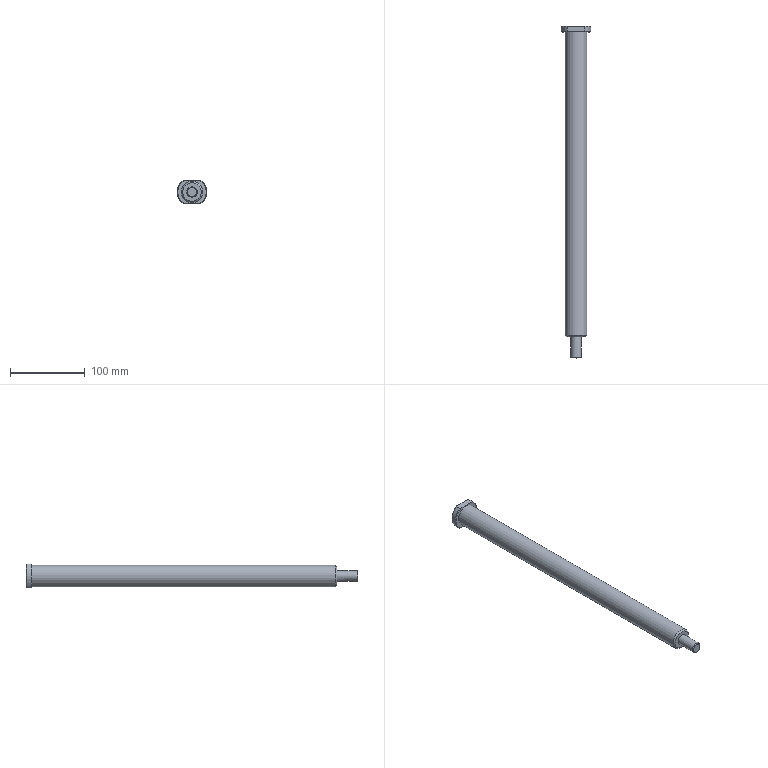Part | STEP file | HL4GZ-1.862.562 (swing arm long shaft) | 1 solid | 16 faces | box 40 x 444.5 x 32 mm | volume 282616 mm3 | plane 6 | cone 6 | cylinder 4 | commonest cylinder face diameters 40 x2 14 x1 29 x1
STEP:
#1=CARTESIAN_POINT('',(0.,0.,0.));
#2=DIRECTION('',(0.,0.,1.));
#3=DIRECTION('',(1.,0.,0.));
#4=AXIS2_PLACEMENT_3D('',#1,#2,#3);
#5=CARTESIAN_POINT('',(1836.876,25.5,-222.582));
#6=VERTEX_POINT('',#5);
#7=CARTESIAN_POINT('',(1838.63,26.5,-222.582));
#8=VERTEX_POINT('',#7);
#9=CARTESIAN_POINT('',(1836.876,25.5,-222.582));
#10=CARTESIAN_POINT('',(1837.451,25.81,-222.582));
#11=CARTESIAN_POINT('',(1838.035,26.143,-222.582));
#12=CARTESIAN_POINT('',(1838.63,26.5,-222.582));
#13=B_SPLINE_CURVE_WITH_KNOTS('',3,(#9,#10,#11,#12),.UNSPECIFIED.,.F.,.F.,(4,4),(0.,1.),.PIECEWISE_BEZIER_KNOTS.);
#14=CARTESIAN_POINT('',(1839.13,36.5,-222.582));
#15=DIRECTION('',(0.,0.,-1.));
#16=DIRECTION('',(1.,0.,0.));
#17=AXIS2_PLACEMENT_3D('',#14,#15,#16);
#18=PLANE('',#17);
#19=CARTESIAN_POINT('',(-2.253,11.));
#20=CARTESIAN_POINT('',(-1.678,10.69));
#21=CARTESIAN_POINT('',(-1.095,10.357));
#22=CARTESIAN_POINT('',(-0.5,10.));
#23=B_SPLINE_CURVE_WITH_KNOTS('',3,(#19,#20,#21,#22),.UNSPECIFIED.,.F.,.F.,(4,4),(0.,1.),.PIECEWISE_BEZIER_KNOTS.);
#24=(GEOMETRIC_REPRESENTATION_CONTEXT(2)PARAMETRIC_REPRESENTATION_CONTEXT()REPRESENTATION_CONTEXT('',''));
#25=DEFINITIONAL_REPRESENTATION('',(#23),#24);
#26=PCURVE('',#18,#25);
#27=CARTESIAN_POINT('',(1826.63,26.,-206.582));
#28=DIRECTION('',(0.,1.,0.));
#29=DIRECTION('',(-0.4067,0.,-0.9135));
#30=AXIS2_PLACEMENT_3D('',#27,#28,#29);
#31=CONICAL_SURFACE('',#30,19.5,0.7854);
#32=CARTESIAN_POINT('',(5.295,-0.5));
#33=CARTESIAN_POINT('',(5.294,-0.4859));
#34=CARTESIAN_POINT('',(5.291,-0.4576));
#35=CARTESIAN_POINT('',(5.288,-0.4149));
#36=CARTESIAN_POINT('',(5.284,-0.3719));
#37=CARTESIAN_POINT('',(5.281,-0.3287));
#38=CARTESIAN_POINT('',(5.277,-0.2851));
#39=CARTESIAN_POINT('',(5.274,-0.2412));
#40=CARTESIAN_POINT('',(5.271,-0.1971));
#41=CARTESIAN_POINT('',(5.267,-0.1526));
#42=CARTESIAN_POINT('',(5.264,-0.1079));
#43=CARTESIAN_POINT('',(5.26,-0.06289));
#44=CARTESIAN_POINT('',(5.257,-0.01758));
#45=CARTESIAN_POINT('',(5.254,0.02802));
#46=CARTESIAN_POINT('',(5.25,0.07391));
#47=CARTESIAN_POINT('',(5.247,0.1201));
#48=CARTESIAN_POINT('',(5.244,0.1666));
#49=CARTESIAN_POINT('',(5.24,0.2133));
#50=CARTESIAN_POINT('',(5.237,0.2604));
#51=CARTESIAN_POINT('',(5.234,0.3077));
#52=CARTESIAN_POINT('',(5.231,0.3553));
#53=CARTESIAN_POINT('',(5.227,0.4032));
#54=CARTESIAN_POINT('',(5.224,0.4515));
#55=CARTESIAN_POINT('',(5.222,0.4838));
#56=CARTESIAN_POINT('',(5.221,0.5));
#57=B_SPLINE_CURVE_WITH_KNOTS('',3,(#32,#33,#34,#35,#36,#37,#38,#39,#40,#41,#42,#43,#44,#45,#46,#47,#48,#49,#50,#51,#52,#53,#54,#55,#56),.UNSPECIFIED.,.F.,.F.,(4,1,1,1,1,1,1,1,1,1,1,1,1,1,1,1,1,1,1,1,1,1,4),(0.,0.04545,0.09091,0.1364,0.1818,0.2273,0.2727,0.3182,0.3636,0.4091,0.4545,0.5,0.5455,0.5909,0.6364,0.6818,0.7273,0.7727,0.8182,0.8636,0.9091,0.9545,1.),.QUASI_UNIFORM_KNOTS.);
#58=(GEOMETRIC_REPRESENTATION_CONTEXT(2)PARAMETRIC_REPRESENTATION_CONTEXT()REPRESENTATION_CONTEXT('',''));
#59=DEFINITIONAL_REPRESENTATION('',(#57),#58);
#60=PCURVE('',#31,#59);
#61=SURFACE_CURVE('',#13,(#26,#60),.PCURVE_S1.);
#62=EDGE_CURVE('',#6,#8,#61,.T.);
#63=ORIENTED_EDGE('',*,*,#62,.F.);
#64=CARTESIAN_POINT('',(1816.383,25.5,-222.582));
#65=VERTEX_POINT('',#64);
#66=CARTESIAN_POINT('',(1826.63,25.5,-222.582));
#67=DIRECTION('',(1.,0.,0.));
#68=VECTOR('',#67,1.);
#69=LINE('',#66,#68);
#70=CARTESIAN_POINT('',(-12.5,11.));
#71=DIRECTION('',(1.,0.));
#72=VECTOR('',#71,1.);
#73=LINE('',#70,#72);
#74=(GEOMETRIC_REPRESENTATION_CONTEXT(2)PARAMETRIC_REPRESENTATION_CONTEXT()REPRESENTATION_CONTEXT('',''));
#75=DEFINITIONAL_REPRESENTATION('',(#73),#74);
#76=PCURVE('',#18,#75);
#77=CARTESIAN_POINT('',(1826.63,25.5,-206.582));
#78=DIRECTION('',(0.,1.,0.));
#79=DIRECTION('',(0.4067,0.,0.9135));
#80=AXIS2_PLACEMENT_3D('',#77,#78,#79);
#81=PLANE('',#80);
#82=CARTESIAN_POINT('',(-14.617,6.508));
#83=DIRECTION('',(0.4067,0.9135));
#84=VECTOR('',#83,1.);
#85=LINE('',#82,#84);
#86=(GEOMETRIC_REPRESENTATION_CONTEXT(2)PARAMETRIC_REPRESENTATION_CONTEXT()REPRESENTATION_CONTEXT('',''));
#87=DEFINITIONAL_REPRESENTATION('',(#85),#86);
#88=PCURVE('',#81,#87);
#89=SURFACE_CURVE('',#69,(#76,#88),.PCURVE_S1.);
#90=EDGE_CURVE('',#65,#6,#89,.T.);
#91=ORIENTED_EDGE('',*,*,#90,.F.);
#92=CARTESIAN_POINT('',(1814.63,26.5,-222.582));
#93=VERTEX_POINT('',#92);
#94=CARTESIAN_POINT('',(1814.63,26.5,-222.582));
#95=CARTESIAN_POINT('',(1815.224,26.143,-222.582));
#96=CARTESIAN_POINT('',(1815.808,25.81,-222.582));
#97=CARTESIAN_POINT('',(1816.383,25.5,-222.582));
#98=B_SPLINE_CURVE_WITH_KNOTS('',3,(#94,#95,#96,#97),.UNSPECIFIED.,.F.,.F.,(4,4),(0.,1.),.PIECEWISE_BEZIER_KNOTS.);
#99=CARTESIAN_POINT('',(-24.5,10.));
#100=CARTESIAN_POINT('',(-23.905,10.357));
#101=CARTESIAN_POINT('',(-23.322,10.69));
#102=CARTESIAN_POINT('',(-22.747,11.));
#103=B_SPLINE_CURVE_WITH_KNOTS('',3,(#99,#100,#101,#102),.UNSPECIFIED.,.F.,.F.,(4,4),(0.,1.),.PIECEWISE_BEZIER_KNOTS.);
#104=(GEOMETRIC_REPRESENTATION_CONTEXT(2)PARAMETRIC_REPRESENTATION_CONTEXT()REPRESENTATION_CONTEXT('',''));
#105=DEFINITIONAL_REPRESENTATION('',(#103),#104);
#106=PCURVE('',#18,#105);
#107=CARTESIAN_POINT('',(1826.63,26.,-206.582));
#108=DIRECTION('',(0.,1.,0.));
#109=DIRECTION('',(-0.4067,0.,-0.9135));
#110=AXIS2_PLACEMENT_3D('',#107,#108,#109);
#111=CONICAL_SURFACE('',#110,19.5,0.7854);
#112=CARTESIAN_POINT('',(0.2246,0.5));
#113=CARTESIAN_POINT('',(0.2235,0.4838));
#114=CARTESIAN_POINT('',(0.2214,0.4515));
#115=CARTESIAN_POINT('',(0.2181,0.4032));
#116=CARTESIAN_POINT('',(0.2148,0.3553));
#117=CARTESIAN_POINT('',(0.2116,0.3077));
#118=CARTESIAN_POINT('',(0.2083,0.2604));
#119=CARTESIAN_POINT('',(0.205,0.2133));
#120=CARTESIAN_POINT('',(0.2017,0.1666));
#121=CARTESIAN_POINT('',(0.1983,0.1201));
#122=CARTESIAN_POINT('',(0.195,0.07391));
#123=CARTESIAN_POINT('',(0.1917,0.02802));
#124=CARTESIAN_POINT('',(0.1883,-0.01758));
#125=CARTESIAN_POINT('',(0.185,-0.06289));
#126=CARTESIAN_POINT('',(0.1816,-0.1079));
#127=CARTESIAN_POINT('',(0.1782,-0.1526));
#128=CARTESIAN_POINT('',(0.1748,-0.1971));
#129=CARTESIAN_POINT('',(0.1714,-0.2412));
#130=CARTESIAN_POINT('',(0.168,-0.2851));
#131=CARTESIAN_POINT('',(0.1646,-0.3287));
#132=CARTESIAN_POINT('',(0.1611,-0.3719));
#133=CARTESIAN_POINT('',(0.1577,-0.4149));
#134=CARTESIAN_POINT('',(0.1542,-0.4576));
#135=CARTESIAN_POINT('',(0.1519,-0.4859));
#136=CARTESIAN_POINT('',(0.1507,-0.5));
#137=B_SPLINE_CURVE_WITH_KNOTS('',3,(#112,#113,#114,#115,#116,#117,#118,#119,#120,#121,#122,#123,#124,#125,#126,#127,#128,#129,#130,#131,#132,#133,#134,#135,#136),.UNSPECIFIED.,.F.,.F.,(4,1,1,1,1,1,1,1,1,1,1,1,1,1,1,1,1,1,1,1,1,1,4),(0.,0.04545,0.09091,0.1364,0.1818,0.2273,0.2727,0.3182,0.3636,0.4091,0.4545,0.5,0.5455,0.5909,0.6364,0.6818,0.7273,0.7727,0.8182,0.8636,0.9091,0.9545,1.),.QUASI_UNIFORM_KNOTS.);
#138=(GEOMETRIC_REPRESENTATION_CONTEXT(2)PARAMETRIC_REPRESENTATION_CONTEXT()REPRESENTATION_CONTEXT('',''));
#139=DEFINITIONAL_REPRESENTATION('',(#137),#138);
#140=PCURVE('',#111,#139);
#141=SURFACE_CURVE('',#98,(#106,#140),.PCURVE_S1.);
#142=EDGE_CURVE('',#93,#65,#141,.T.);
#143=ORIENTED_EDGE('',*,*,#142,.F.);
#144=CARTESIAN_POINT('',(1814.63,32.5,-222.582));
#145=VERTEX_POINT('',#144);
#146=CARTESIAN_POINT('',(1814.63,25.5,-222.582));
#147=DIRECTION('',(0.,-1.,0.));
#148=VECTOR('',#147,1.);
#149=LINE('',#146,#148);
#150=CARTESIAN_POINT('',(-24.5,11.));
#151=DIRECTION('',(0.,1.));
#152=VECTOR('',#151,1.);
#153=LINE('',#150,#152);
#154=(GEOMETRIC_REPRESENTATION_CONTEXT(2)PARAMETRIC_REPRESENTATION_CONTEXT()REPRESENTATION_CONTEXT('',''));
#155=DEFINITIONAL_REPRESENTATION('',(#153),#154);
#156=PCURVE('',#18,#155);
#157=CARTESIAN_POINT('',(1826.63,25.5,-206.582));
#158=DIRECTION('',(0.,1.,0.));
#159=DIRECTION('',(-0.4067,0.,-0.9135));
#160=AXIS2_PLACEMENT_3D('',#157,#158,#159);
#161=CYLINDRICAL_SURFACE('',#160,20.);
#162=CARTESIAN_POINT('',(0.2246,0.));
#163=DIRECTION('',(0.,-1.));
#164=VECTOR('',#163,1.);
#165=LINE('',#162,#164);
#166=(GEOMETRIC_REPRESENTATION_CONTEXT(2)PARAMETRIC_REPRESENTATION_CONTEXT()REPRESENTATION_CONTEXT('',''));
#167=DEFINITIONAL_REPRESENTATION('',(#165),#166);
#168=PCURVE('',#161,#167);
#169=SURFACE_CURVE('',#149,(#156,#168),.PCURVE_S1.);
#170=EDGE_CURVE('',#145,#93,#169,.T.);
#171=ORIENTED_EDGE('',*,*,#170,.F.);
#172=CARTESIAN_POINT('',(1816.383,33.5,-222.582));
#173=VERTEX_POINT('',#172);
#174=CARTESIAN_POINT('',(1816.383,33.5,-222.582));
#175=CARTESIAN_POINT('',(1815.808,33.19,-222.582));
#176=CARTESIAN_POINT('',(1815.224,32.857,-222.582));
#177=CARTESIAN_POINT('',(1814.63,32.5,-222.582));
#178=B_SPLINE_CURVE_WITH_KNOTS('',3,(#174,#175,#176,#177),.UNSPECIFIED.,.F.,.F.,(4,4),(0.,1.),.PIECEWISE_BEZIER_KNOTS.);
#179=CARTESIAN_POINT('',(-22.747,3.));
#180=CARTESIAN_POINT('',(-23.322,3.31));
#181=CARTESIAN_POINT('',(-23.905,3.643));
#182=CARTESIAN_POINT('',(-24.5,4.));
#183=B_SPLINE_CURVE_WITH_KNOTS('',3,(#179,#180,#181,#182),.UNSPECIFIED.,.F.,.F.,(4,4),(0.,1.),.PIECEWISE_BEZIER_KNOTS.);
#184=(GEOMETRIC_REPRESENTATION_CONTEXT(2)PARAMETRIC_REPRESENTATION_CONTEXT()REPRESENTATION_CONTEXT('',''));
#185=DEFINITIONAL_REPRESENTATION('',(#183),#184);
#186=PCURVE('',#18,#185);
#187=CARTESIAN_POINT('',(1826.63,33.,-206.582));
#188=DIRECTION('',(0.,-1.,0.));
#189=DIRECTION('',(-0.4067,0.,-0.9135));
#190=AXIS2_PLACEMENT_3D('',#187,#188,#189);
#191=CONICAL_SURFACE('',#190,19.5,0.7854);
#192=CARTESIAN_POINT('',(6.132,-0.5));
#193=CARTESIAN_POINT('',(6.131,-0.4859));
#194=CARTESIAN_POINT('',(6.129,-0.4576));
#195=CARTESIAN_POINT('',(6.126,-0.4149));
#196=CARTESIAN_POINT('',(6.122,-0.3719));
#197=CARTESIAN_POINT('',(6.119,-0.3287));
#198=CARTESIAN_POINT('',(6.115,-0.2851));
#199=CARTESIAN_POINT('',(6.112,-0.2412));
#200=CARTESIAN_POINT('',(6.108,-0.1971));
#201=CARTESIAN_POINT('',(6.105,-0.1526));
#202=CARTESIAN_POINT('',(6.102,-0.1079));
#203=CARTESIAN_POINT('',(6.098,-0.06289));
#204=CARTESIAN_POINT('',(6.095,-0.01758));
#205=CARTESIAN_POINT('',(6.092,0.02802));
#206=CARTESIAN_POINT('',(6.088,0.07391));
#207=CARTESIAN_POINT('',(6.085,0.1201));
#208=CARTESIAN_POINT('',(6.082,0.1666));
#209=CARTESIAN_POINT('',(6.078,0.2133));
#210=CARTESIAN_POINT('',(6.075,0.2604));
#211=CARTESIAN_POINT('',(6.072,0.3077));
#212=CARTESIAN_POINT('',(6.068,0.3553));
#213=CARTESIAN_POINT('',(6.065,0.4032));
#214=CARTESIAN_POINT('',(6.062,0.4515));
#215=CARTESIAN_POINT('',(6.06,0.4838));
#216=CARTESIAN_POINT('',(6.059,0.5));
#217=B_SPLINE_CURVE_WITH_KNOTS('',3,(#192,#193,#194,#195,#196,#197,#198,#199,#200,#201,#202,#203,#204,#205,#206,#207,#208,#209,#210,#211,#212,#213,#214,#215,#216),.UNSPECIFIED.,.F.,.F.,(4,1,1,1,1,1,1,1,1,1,1,1,1,1,1,1,1,1,1,1,1,1,4),(0.,0.04545,0.09091,0.1364,0.1818,0.2273,0.2727,0.3182,0.3636,0.4091,0.4545,0.5,0.5455,0.5909,0.6364,0.6818,0.7273,0.7727,0.8182,0.8636,0.9091,0.9545,1.),.QUASI_UNIFORM_KNOTS.);
#218=(GEOMETRIC_REPRESENTATION_CONTEXT(2)PARAMETRIC_REPRESENTATION_CONTEXT()REPRESENTATION_CONTEXT('',''));
#219=DEFINITIONAL_REPRESENTATION('',(#217),#218);
#220=PCURVE('',#191,#219);
#221=SURFACE_CURVE('',#178,(#186,#220),.PCURVE_S1.);
#222=EDGE_CURVE('',#173,#145,#221,.T.);
#223=ORIENTED_EDGE('',*,*,#222,.F.);
#224=CARTESIAN_POINT('',(1836.876,33.5,-222.582));
#225=VERTEX_POINT('',#224);
#226=CARTESIAN_POINT('',(1826.63,33.5,-222.582));
#227=DIRECTION('',(1.,0.,0.));
#228=VECTOR('',#227,1.);
#229=LINE('',#226,#228);
#230=CARTESIAN_POINT('',(-12.5,3.));
#231=DIRECTION('',(1.,0.));
#232=VECTOR('',#231,1.);
#233=LINE('',#230,#232);
#234=(GEOMETRIC_REPRESENTATION_CONTEXT(2)PARAMETRIC_REPRESENTATION_CONTEXT()REPRESENTATION_CONTEXT('',''));
#235=DEFINITIONAL_REPRESENTATION('',(#233),#234);
#236=PCURVE('',#18,#235);
#237=CARTESIAN_POINT('',(1826.63,33.5,-206.582));
#238=DIRECTION('',(0.,1.,0.));
#239=DIRECTION('',(0.4067,0.,0.9135));
#240=AXIS2_PLACEMENT_3D('',#237,#238,#239);
#241=PLANE('',#240);
#242=CARTESIAN_POINT('',(-14.617,6.508));
#243=DIRECTION('',(0.4067,0.9135));
#244=VECTOR('',#243,1.);
#245=LINE('',#242,#244);
#246=(GEOMETRIC_REPRESENTATION_CONTEXT(2)PARAMETRIC_REPRESENTATION_CONTEXT()REPRESENTATION_CONTEXT('',''));
#247=DEFINITIONAL_REPRESENTATION('',(#245),#246);
#248=PCURVE('',#241,#247);
#249=SURFACE_CURVE('',#229,(#236,#248),.PCURVE_S1.);
#250=EDGE_CURVE('',#173,#225,#249,.T.);
#251=ORIENTED_EDGE('',*,*,#250,.T.);
#252=CARTESIAN_POINT('',(1838.63,32.5,-222.582));
#253=VERTEX_POINT('',#252);
#254=CARTESIAN_POINT('',(1838.63,32.5,-222.582));
#255=CARTESIAN_POINT('',(1838.035,32.857,-222.582));
#256=CARTESIAN_POINT('',(1837.451,33.19,-222.582));
#257=CARTESIAN_POINT('',(1836.876,33.5,-222.582));
#258=B_SPLINE_CURVE_WITH_KNOTS('',3,(#254,#255,#256,#257),.UNSPECIFIED.,.F.,.F.,(4,4),(0.,1.),.PIECEWISE_BEZIER_KNOTS.);
#259=CARTESIAN_POINT('',(-0.5,4.));
#260=CARTESIAN_POINT('',(-1.095,3.643));
#261=CARTESIAN_POINT('',(-1.678,3.31));
#262=CARTESIAN_POINT('',(-2.253,3.));
#263=B_SPLINE_CURVE_WITH_KNOTS('',3,(#259,#260,#261,#262),.UNSPECIFIED.,.F.,.F.,(4,4),(0.,1.),.PIECEWISE_BEZIER_KNOTS.);
#264=(GEOMETRIC_REPRESENTATION_CONTEXT(2)PARAMETRIC_REPRESENTATION_CONTEXT()REPRESENTATION_CONTEXT('',''));
#265=DEFINITIONAL_REPRESENTATION('',(#263),#264);
#266=PCURVE('',#18,#265);
#267=CARTESIAN_POINT('',(1826.63,33.,-206.582));
#268=DIRECTION('',(0.,-1.,0.));
#269=DIRECTION('',(-0.4067,0.,-0.9135));
#270=AXIS2_PLACEMENT_3D('',#267,#268,#269);
#271=CONICAL_SURFACE('',#270,19.5,0.7854);
#272=CARTESIAN_POINT('',(1.062,0.5));
#273=CARTESIAN_POINT('',(1.061,0.4838));
#274=CARTESIAN_POINT('',(1.059,0.4515));
#275=CARTESIAN_POINT('',(1.056,0.4032));
#276=CARTESIAN_POINT('',(1.053,0.3553));
#277=CARTESIAN_POINT('',(1.049,0.3077));
#278=CARTESIAN_POINT('',(1.046,0.2604));
#279=CARTESIAN_POINT('',(1.043,0.2133));
#280=CARTESIAN_POINT('',(1.039,0.1666));
#281=CARTESIAN_POINT('',(1.036,0.1201));
#282=CARTESIAN_POINT('',(1.033,0.07391));
#283=CARTESIAN_POINT('',(1.029,0.02802));
#284=CARTESIAN_POINT('',(1.026,-0.01758));
#285=CARTESIAN_POINT('',(1.023,-0.06289));
#286=CARTESIAN_POINT('',(1.019,-0.1079));
#287=CARTESIAN_POINT('',(1.016,-0.1526));
#288=CARTESIAN_POINT('',(1.013,-0.1971));
#289=CARTESIAN_POINT('',(1.009,-0.2412));
#290=CARTESIAN_POINT('',(1.006,-0.2851));
#291=CARTESIAN_POINT('',(1.002,-0.3287));
#292=CARTESIAN_POINT('',(0.9989,-0.3719));
#293=CARTESIAN_POINT('',(0.9954,-0.4149));
#294=CARTESIAN_POINT('',(0.992,-0.4576));
#295=CARTESIAN_POINT('',(0.9897,-0.4859));
#296=CARTESIAN_POINT('',(0.9885,-0.5));
#297=B_SPLINE_CURVE_WITH_KNOTS('',3,(#272,#273,#274,#275,#276,#277,#278,#279,#280,#281,#282,#283,#284,#285,#286,#287,#288,#289,#290,#291,#292,#293,#294,#295,#296),.UNSPECIFIED.,.F.,.F.,(4,1,1,1,1,1,1,1,1,1,1,1,1,1,1,1,1,1,1,1,1,1,4),(0.,0.04545,0.09091,0.1364,0.1818,0.2273,0.2727,0.3182,0.3636,0.4091,0.4545,0.5,0.5455,0.5909,0.6364,0.6818,0.7273,0.7727,0.8182,0.8636,0.9091,0.9545,1.),.QUASI_UNIFORM_KNOTS.);
#298=(GEOMETRIC_REPRESENTATION_CONTEXT(2)PARAMETRIC_REPRESENTATION_CONTEXT()REPRESENTATION_CONTEXT('',''));
#299=DEFINITIONAL_REPRESENTATION('',(#297),#298);
#300=PCURVE('',#271,#299);
#301=SURFACE_CURVE('',#258,(#266,#300),.PCURVE_S1.);
#302=EDGE_CURVE('',#253,#225,#301,.T.);
#303=ORIENTED_EDGE('',*,*,#302,.F.);
#304=CARTESIAN_POINT('',(1838.63,25.5,-222.582));
#305=DIRECTION('',(0.,1.,0.));
#306=VECTOR('',#305,1.);
#307=LINE('',#304,#306);
#308=CARTESIAN_POINT('',(-0.5,11.));
#309=DIRECTION('',(0.,-1.));
#310=VECTOR('',#309,1.);
#311=LINE('',#308,#310);
#312=(GEOMETRIC_REPRESENTATION_CONTEXT(2)PARAMETRIC_REPRESENTATION_CONTEXT()REPRESENTATION_CONTEXT('',''));
#313=DEFINITIONAL_REPRESENTATION('',(#311),#312);
#314=PCURVE('',#18,#313);
#315=CARTESIAN_POINT('',(1826.63,25.5,-206.582));
#316=DIRECTION('',(0.,1.,0.));
#317=DIRECTION('',(-0.4067,0.,-0.9135));
#318=AXIS2_PLACEMENT_3D('',#315,#316,#317);
#319=CYLINDRICAL_SURFACE('',#318,20.);
#320=CARTESIAN_POINT('',(5.221,0.));
#321=DIRECTION('',(0.,1.));
#322=VECTOR('',#321,1.);
#323=LINE('',#320,#322);
#324=(GEOMETRIC_REPRESENTATION_CONTEXT(2)PARAMETRIC_REPRESENTATION_CONTEXT()REPRESENTATION_CONTEXT('',''));
#325=DEFINITIONAL_REPRESENTATION('',(#323),#324);
#326=PCURVE('',#319,#325);
#327=SURFACE_CURVE('',#307,(#314,#326),.PCURVE_S1.);
#328=EDGE_CURVE('',#8,#253,#327,.T.);
#329=ORIENTED_EDGE('',*,*,#328,.F.);
#330=EDGE_LOOP('',(#63,#91,#143,#171,#223,#251,#303,#329));
#331=FACE_BOUND('',#330,.T.);
#332=ADVANCED_FACE('',(#331),#18,.T.);
#333=CARTESIAN_POINT('',(1838.63,26.5,-190.582));
#334=VERTEX_POINT('',#333);
#335=CARTESIAN_POINT('',(1836.876,25.5,-190.582));
#336=VERTEX_POINT('',#335);
#337=CARTESIAN_POINT('',(1838.63,26.5,-190.582));
#338=CARTESIAN_POINT('',(1838.035,26.143,-190.582));
#339=CARTESIAN_POINT('',(1837.451,25.81,-190.582));
#340=CARTESIAN_POINT('',(1836.876,25.5,-190.582));
#341=B_SPLINE_CURVE_WITH_KNOTS('',3,(#337,#338,#339,#340),.UNSPECIFIED.,.F.,.F.,(4,4),(0.,1.),.PIECEWISE_BEZIER_KNOTS.);
#342=CARTESIAN_POINT('',(1839.13,36.5,-190.582));
#343=DIRECTION('',(0.,0.,-1.));
#344=DIRECTION('',(1.,0.,0.));
#345=AXIS2_PLACEMENT_3D('',#342,#343,#344);
#346=PLANE('',#345);
#347=CARTESIAN_POINT('',(-0.5,10.));
#348=CARTESIAN_POINT('',(-1.095,10.357));
#349=CARTESIAN_POINT('',(-1.678,10.69));
#350=CARTESIAN_POINT('',(-2.253,11.));
#351=B_SPLINE_CURVE_WITH_KNOTS('',3,(#347,#348,#349,#350),.UNSPECIFIED.,.F.,.F.,(4,4),(0.,1.),.PIECEWISE_BEZIER_KNOTS.);
#352=(GEOMETRIC_REPRESENTATION_CONTEXT(2)PARAMETRIC_REPRESENTATION_CONTEXT()REPRESENTATION_CONTEXT('',''));
#353=DEFINITIONAL_REPRESENTATION('',(#351),#352);
#354=PCURVE('',#346,#353);
#355=CARTESIAN_POINT('',(3.366,0.5));
#356=CARTESIAN_POINT('',(3.365,0.4838));
#357=CARTESIAN_POINT('',(3.363,0.4515));
#358=CARTESIAN_POINT('',(3.36,0.4032));
#359=CARTESIAN_POINT('',(3.356,0.3553));
#360=CARTESIAN_POINT('',(3.353,0.3077));
#361=CARTESIAN_POINT('',(3.35,0.2604));
#362=CARTESIAN_POINT('',(3.347,0.2133));
#363=CARTESIAN_POINT('',(3.343,0.1666));
#364=CARTESIAN_POINT('',(3.34,0.1201));
#365=CARTESIAN_POINT('',(3.337,0.07391));
#366=CARTESIAN_POINT('',(3.333,0.02802));
#367=CARTESIAN_POINT('',(3.33,-0.01758));
#368=CARTESIAN_POINT('',(3.327,-0.06289));
#369=CARTESIAN_POINT('',(3.323,-0.1079));
#370=CARTESIAN_POINT('',(3.32,-0.1526));
#371=CARTESIAN_POINT('',(3.316,-0.1971));
#372=CARTESIAN_POINT('',(3.313,-0.2412));
#373=CARTESIAN_POINT('',(3.31,-0.2851));
#374=CARTESIAN_POINT('',(3.306,-0.3287));
#375=CARTESIAN_POINT('',(3.303,-0.3719));
#376=CARTESIAN_POINT('',(3.299,-0.4149));
#377=CARTESIAN_POINT('',(3.296,-0.4576));
#378=CARTESIAN_POINT('',(3.293,-0.4859));
#379=CARTESIAN_POINT('',(3.292,-0.5));
#380=B_SPLINE_CURVE_WITH_KNOTS('',3,(#355,#356,#357,#358,#359,#360,#361,#362,#363,#364,#365,#366,#367,#368,#369,#370,#371,#372,#373,#374,#375,#376,#377,#378,#379),.UNSPECIFIED.,.F.,.F.,(4,1,1,1,1,1,1,1,1,1,1,1,1,1,1,1,1,1,1,1,1,1,4),(0.,0.04545,0.09091,0.1364,0.1818,0.2273,0.2727,0.3182,0.3636,0.4091,0.4545,0.5,0.5455,0.5909,0.6364,0.6818,0.7273,0.7727,0.8182,0.8636,0.9091,0.9545,1.),.QUASI_UNIFORM_KNOTS.);
#381=(GEOMETRIC_REPRESENTATION_CONTEXT(2)PARAMETRIC_REPRESENTATION_CONTEXT()REPRESENTATION_CONTEXT('',''));
#382=DEFINITIONAL_REPRESENTATION('',(#380),#381);
#383=PCURVE('',#31,#382);
#384=SURFACE_CURVE('',#341,(#354,#383),.PCURVE_S1.);
#385=EDGE_CURVE('',#334,#336,#384,.T.);
#386=ORIENTED_EDGE('',*,*,#385,.F.);
#387=CARTESIAN_POINT('',(1838.63,32.5,-190.582));
#388=VERTEX_POINT('',#387);
#389=CARTESIAN_POINT('',(1838.63,25.5,-190.582));
#390=DIRECTION('',(0.,-1.,0.));
#391=VECTOR('',#390,1.);
#392=LINE('',#389,#391);
#393=CARTESIAN_POINT('',(-0.5,11.));
#394=DIRECTION('',(0.,1.));
#395=VECTOR('',#394,1.);
#396=LINE('',#393,#395);
#397=(GEOMETRIC_REPRESENTATION_CONTEXT(2)PARAMETRIC_REPRESENTATION_CONTEXT()REPRESENTATION_CONTEXT('',''));
#398=DEFINITIONAL_REPRESENTATION('',(#396),#397);
#399=PCURVE('',#346,#398);
#400=CARTESIAN_POINT('',(3.366,0.));
#401=DIRECTION('',(0.,-1.));
#402=VECTOR('',#401,1.);
#403=LINE('',#400,#402);
#404=(GEOMETRIC_REPRESENTATION_CONTEXT(2)PARAMETRIC_REPRESENTATION_CONTEXT()REPRESENTATION_CONTEXT('',''));
#405=DEFINITIONAL_REPRESENTATION('',(#403),#404);
#406=PCURVE('',#319,#405);
#407=SURFACE_CURVE('',#392,(#399,#406),.PCURVE_S1.);
#408=EDGE_CURVE('',#388,#334,#407,.T.);
#409=ORIENTED_EDGE('',*,*,#408,.F.);
#410=CARTESIAN_POINT('',(1836.876,33.5,-190.582));
#411=VERTEX_POINT('',#410);
#412=CARTESIAN_POINT('',(1836.876,33.5,-190.582));
#413=CARTESIAN_POINT('',(1837.451,33.19,-190.582));
#414=CARTESIAN_POINT('',(1838.035,32.857,-190.582));
#415=CARTESIAN_POINT('',(1838.63,32.5,-190.582));
#416=B_SPLINE_CURVE_WITH_KNOTS('',3,(#412,#413,#414,#415),.UNSPECIFIED.,.F.,.F.,(4,4),(0.,1.),.PIECEWISE_BEZIER_KNOTS.);
#417=CARTESIAN_POINT('',(-2.253,3.));
#418=CARTESIAN_POINT('',(-1.678,3.31));
#419=CARTESIAN_POINT('',(-1.095,3.643));
#420=CARTESIAN_POINT('',(-0.5,4.));
#421=B_SPLINE_CURVE_WITH_KNOTS('',3,(#417,#418,#419,#420),.UNSPECIFIED.,.F.,.F.,(4,4),(0.,1.),.PIECEWISE_BEZIER_KNOTS.);
#422=(GEOMETRIC_REPRESENTATION_CONTEXT(2)PARAMETRIC_REPRESENTATION_CONTEXT()REPRESENTATION_CONTEXT('',''));
#423=DEFINITIONAL_REPRESENTATION('',(#421),#422);
#424=PCURVE('',#346,#423);
#425=CARTESIAN_POINT('',(2.991,-0.5));
#426=CARTESIAN_POINT('',(2.99,-0.4859));
#427=CARTESIAN_POINT('',(2.987,-0.4576));
#428=CARTESIAN_POINT('',(2.984,-0.4149));
#429=CARTESIAN_POINT('',(2.98,-0.3719));
#430=CARTESIAN_POINT('',(2.977,-0.3287));
#431=CARTESIAN_POINT('',(2.974,-0.2851));
#432=CARTESIAN_POINT('',(2.97,-0.2412));
#433=CARTESIAN_POINT('',(2.967,-0.1971));
#434=CARTESIAN_POINT('',(2.963,-0.1526));
#435=CARTESIAN_POINT('',(2.96,-0.1079));
#436=CARTESIAN_POINT('',(2.957,-0.06289));
#437=CARTESIAN_POINT('',(2.953,-0.01758));
#438=CARTESIAN_POINT('',(2.95,0.02802));
#439=CARTESIAN_POINT('',(2.947,0.07391));
#440=CARTESIAN_POINT('',(2.943,0.1201));
#441=CARTESIAN_POINT('',(2.94,0.1666));
#442=CARTESIAN_POINT('',(2.937,0.2133));
#443=CARTESIAN_POINT('',(2.933,0.2604));
#444=CARTESIAN_POINT('',(2.93,0.3077));
#445=CARTESIAN_POINT('',(2.927,0.3553));
#446=CARTESIAN_POINT('',(2.923,0.4032));
#447=CARTESIAN_POINT('',(2.92,0.4515));
#448=CARTESIAN_POINT('',(2.918,0.4838));
#449=CARTESIAN_POINT('',(2.917,0.5));
#450=B_SPLINE_CURVE_WITH_KNOTS('',3,(#425,#426,#427,#428,#429,#430,#431,#432,#433,#434,#435,#436,#437,#438,#439,#440,#441,#442,#443,#444,#445,#446,#447,#448,#449),.UNSPECIFIED.,.F.,.F.,(4,1,1,1,1,1,1,1,1,1,1,1,1,1,1,1,1,1,1,1,1,1,4),(0.,0.04545,0.09091,0.1364,0.1818,0.2273,0.2727,0.3182,0.3636,0.4091,0.4545,0.5,0.5455,0.5909,0.6364,0.6818,0.7273,0.7727,0.8182,0.8636,0.9091,0.9545,1.),.QUASI_UNIFORM_KNOTS.);
#451=(GEOMETRIC_REPRESENTATION_CONTEXT(2)PARAMETRIC_REPRESENTATION_CONTEXT()REPRESENTATION_CONTEXT('',''));
#452=DEFINITIONAL_REPRESENTATION('',(#450),#451);
#453=PCURVE('',#271,#452);
#454=SURFACE_CURVE('',#416,(#424,#453),.PCURVE_S1.);
#455=EDGE_CURVE('',#411,#388,#454,.T.);
#456=ORIENTED_EDGE('',*,*,#455,.F.);
#457=CARTESIAN_POINT('',(1816.383,33.5,-190.582));
#458=VERTEX_POINT('',#457);
#459=CARTESIAN_POINT('',(1826.63,33.5,-190.582));
#460=DIRECTION('',(1.,0.,0.));
#461=VECTOR('',#460,1.);
#462=LINE('',#459,#461);
#463=CARTESIAN_POINT('',(-12.5,3.));
#464=DIRECTION('',(1.,0.));
#465=VECTOR('',#464,1.);
#466=LINE('',#463,#465);
#467=(GEOMETRIC_REPRESENTATION_CONTEXT(2)PARAMETRIC_REPRESENTATION_CONTEXT()REPRESENTATION_CONTEXT('',''));
#468=DEFINITIONAL_REPRESENTATION('',(#466),#467);
#469=PCURVE('',#346,#468);
#470=CARTESIAN_POINT('',(14.617,-6.508));
#471=DIRECTION('',(0.4067,0.9135));
#472=VECTOR('',#471,1.);
#473=LINE('',#470,#472);
#474=(GEOMETRIC_REPRESENTATION_CONTEXT(2)PARAMETRIC_REPRESENTATION_CONTEXT()REPRESENTATION_CONTEXT('',''));
#475=DEFINITIONAL_REPRESENTATION('',(#473),#474);
#476=PCURVE('',#241,#475);
#477=SURFACE_CURVE('',#462,(#469,#476),.PCURVE_S1.);
#478=EDGE_CURVE('',#458,#411,#477,.T.);
#479=ORIENTED_EDGE('',*,*,#478,.F.);
#480=CARTESIAN_POINT('',(1814.63,32.5,-190.582));
#481=VERTEX_POINT('',#480);
#482=CARTESIAN_POINT('',(1814.63,32.5,-190.582));
#483=CARTESIAN_POINT('',(1815.224,32.857,-190.582));
#484=CARTESIAN_POINT('',(1815.808,33.19,-190.582));
#485=CARTESIAN_POINT('',(1816.383,33.5,-190.582));
#486=B_SPLINE_CURVE_WITH_KNOTS('',3,(#482,#483,#484,#485),.UNSPECIFIED.,.F.,.F.,(4,4),(0.,1.),.PIECEWISE_BEZIER_KNOTS.);
#487=CARTESIAN_POINT('',(-24.5,4.));
#488=CARTESIAN_POINT('',(-23.905,3.643));
#489=CARTESIAN_POINT('',(-23.322,3.31));
#490=CARTESIAN_POINT('',(-22.747,3.));
#491=B_SPLINE_CURVE_WITH_KNOTS('',3,(#487,#488,#489,#490),.UNSPECIFIED.,.F.,.F.,(4,4),(0.,1.),.PIECEWISE_BEZIER_KNOTS.);
#492=(GEOMETRIC_REPRESENTATION_CONTEXT(2)PARAMETRIC_REPRESENTATION_CONTEXT()REPRESENTATION_CONTEXT('',''));
#493=DEFINITIONAL_REPRESENTATION('',(#491),#492);
#494=PCURVE('',#346,#493);
#495=CARTESIAN_POINT('',(4.204,0.5));
#496=CARTESIAN_POINT('',(4.203,0.4838));
#497=CARTESIAN_POINT('',(4.201,0.4515));
#498=CARTESIAN_POINT('',(4.197,0.4032));
#499=CARTESIAN_POINT('',(4.194,0.3553));
#500=CARTESIAN_POINT('',(4.191,0.3077));
#501=CARTESIAN_POINT('',(4.188,0.2604));
#502=CARTESIAN_POINT('',(4.184,0.2133));
#503=CARTESIAN_POINT('',(4.181,0.1666));
#504=CARTESIAN_POINT('',(4.178,0.1201));
#505=CARTESIAN_POINT('',(4.174,0.07391));
#506=CARTESIAN_POINT('',(4.171,0.02802));
#507=CARTESIAN_POINT('',(4.168,-0.01758));
#508=CARTESIAN_POINT('',(4.164,-0.06289));
#509=CARTESIAN_POINT('',(4.161,-0.1079));
#510=CARTESIAN_POINT('',(4.158,-0.1526));
#511=CARTESIAN_POINT('',(4.154,-0.1971));
#512=CARTESIAN_POINT('',(4.151,-0.2412));
#513=CARTESIAN_POINT('',(4.147,-0.2851));
#514=CARTESIAN_POINT('',(4.144,-0.3287));
#515=CARTESIAN_POINT('',(4.14,-0.3719));
#516=CARTESIAN_POINT('',(4.137,-0.4149));
#517=CARTESIAN_POINT('',(4.134,-0.4576));
#518=CARTESIAN_POINT('',(4.131,-0.4859));
#519=CARTESIAN_POINT('',(4.13,-0.5));
#520=B_SPLINE_CURVE_WITH_KNOTS('',3,(#495,#496,#497,#498,#499,#500,#501,#502,#503,#504,#505,#506,#507,#508,#509,#510,#511,#512,#513,#514,#515,#516,#517,#518,#519),.UNSPECIFIED.,.F.,.F.,(4,1,1,1,1,1,1,1,1,1,1,1,1,1,1,1,1,1,1,1,1,1,4),(0.,0.04545,0.09091,0.1364,0.1818,0.2273,0.2727,0.3182,0.3636,0.4091,0.4545,0.5,0.5455,0.5909,0.6364,0.6818,0.7273,0.7727,0.8182,0.8636,0.9091,0.9545,1.),.QUASI_UNIFORM_KNOTS.);
#521=(GEOMETRIC_REPRESENTATION_CONTEXT(2)PARAMETRIC_REPRESENTATION_CONTEXT()REPRESENTATION_CONTEXT('',''));
#522=DEFINITIONAL_REPRESENTATION('',(#520),#521);
#523=PCURVE('',#191,#522);
#524=SURFACE_CURVE('',#486,(#494,#523),.PCURVE_S1.);
#525=EDGE_CURVE('',#481,#458,#524,.T.);
#526=ORIENTED_EDGE('',*,*,#525,.F.);
#527=CARTESIAN_POINT('',(1814.63,26.5,-190.582));
#528=VERTEX_POINT('',#527);
#529=CARTESIAN_POINT('',(1814.63,25.5,-190.582));
#530=DIRECTION('',(0.,1.,0.));
#531=VECTOR('',#530,1.);
#532=LINE('',#529,#531);
#533=CARTESIAN_POINT('',(-24.5,11.));
#534=DIRECTION('',(0.,-1.));
#535=VECTOR('',#534,1.);
#536=LINE('',#533,#535);
#537=(GEOMETRIC_REPRESENTATION_CONTEXT(2)PARAMETRIC_REPRESENTATION_CONTEXT()REPRESENTATION_CONTEXT('',''));
#538=DEFINITIONAL_REPRESENTATION('',(#536),#537);
#539=PCURVE('',#346,#538);
#540=CARTESIAN_POINT('',(2.079,0.));
#541=DIRECTION('',(0.,1.));
#542=VECTOR('',#541,1.);
#543=LINE('',#540,#542);
#544=(GEOMETRIC_REPRESENTATION_CONTEXT(2)PARAMETRIC_REPRESENTATION_CONTEXT()REPRESENTATION_CONTEXT('',''));
#545=DEFINITIONAL_REPRESENTATION('',(#543),#544);
#546=PCURVE('',#161,#545);
#547=SURFACE_CURVE('',#532,(#539,#546),.PCURVE_S1.);
#548=EDGE_CURVE('',#528,#481,#547,.T.);
#549=ORIENTED_EDGE('',*,*,#548,.F.);
#550=CARTESIAN_POINT('',(1816.383,25.5,-190.582));
#551=VERTEX_POINT('',#550);
#552=CARTESIAN_POINT('',(1816.383,25.5,-190.582));
#553=CARTESIAN_POINT('',(1815.808,25.81,-190.582));
#554=CARTESIAN_POINT('',(1815.224,26.143,-190.582));
#555=CARTESIAN_POINT('',(1814.63,26.5,-190.582));
#556=B_SPLINE_CURVE_WITH_KNOTS('',3,(#552,#553,#554,#555),.UNSPECIFIED.,.F.,.F.,(4,4),(0.,1.),.PIECEWISE_BEZIER_KNOTS.);
#557=CARTESIAN_POINT('',(-22.747,11.));
#558=CARTESIAN_POINT('',(-23.322,10.69));
#559=CARTESIAN_POINT('',(-23.905,10.357));
#560=CARTESIAN_POINT('',(-24.5,10.));
#561=B_SPLINE_CURVE_WITH_KNOTS('',3,(#557,#558,#559,#560),.UNSPECIFIED.,.F.,.F.,(4,4),(0.,1.),.PIECEWISE_BEZIER_KNOTS.);
#562=(GEOMETRIC_REPRESENTATION_CONTEXT(2)PARAMETRIC_REPRESENTATION_CONTEXT()REPRESENTATION_CONTEXT('',''));
#563=DEFINITIONAL_REPRESENTATION('',(#561),#562);
#564=PCURVE('',#346,#563);
#565=CARTESIAN_POINT('',(2.153,-0.5));
#566=CARTESIAN_POINT('',(2.152,-0.4859));
#567=CARTESIAN_POINT('',(2.15,-0.4576));
#568=CARTESIAN_POINT('',(2.146,-0.4149));
#569=CARTESIAN_POINT('',(2.143,-0.3719));
#570=CARTESIAN_POINT('',(2.139,-0.3287));
#571=CARTESIAN_POINT('',(2.136,-0.2851));
#572=CARTESIAN_POINT('',(2.132,-0.2412));
#573=CARTESIAN_POINT('',(2.129,-0.1971));
#574=CARTESIAN_POINT('',(2.126,-0.1526));
#575=CARTESIAN_POINT('',(2.122,-0.1079));
#576=CARTESIAN_POINT('',(2.119,-0.06289));
#577=CARTESIAN_POINT('',(2.116,-0.01758));
#578=CARTESIAN_POINT('',(2.112,0.02802));
#579=CARTESIAN_POINT('',(2.109,0.07391));
#580=CARTESIAN_POINT('',(2.105,0.1201));
#581=CARTESIAN_POINT('',(2.102,0.1666));
#582=CARTESIAN_POINT('',(2.099,0.2133));
#583=CARTESIAN_POINT('',(2.096,0.2604));
#584=CARTESIAN_POINT('',(2.092,0.3077));
#585=CARTESIAN_POINT('',(2.089,0.3553));
#586=CARTESIAN_POINT('',(2.086,0.4032));
#587=CARTESIAN_POINT('',(2.082,0.4515));
#588=CARTESIAN_POINT('',(2.08,0.4838));
#589=CARTESIAN_POINT('',(2.079,0.5));
#590=B_SPLINE_CURVE_WITH_KNOTS('',3,(#565,#566,#567,#568,#569,#570,#571,#572,#573,#574,#575,#576,#577,#578,#579,#580,#581,#582,#583,#584,#585,#586,#587,#588,#589),.UNSPECIFIED.,.F.,.F.,(4,1,1,1,1,1,1,1,1,1,1,1,1,1,1,1,1,1,1,1,1,1,4),(0.,0.04545,0.09091,0.1364,0.1818,0.2273,0.2727,0.3182,0.3636,0.4091,0.4545,0.5,0.5455,0.5909,0.6364,0.6818,0.7273,0.7727,0.8182,0.8636,0.9091,0.9545,1.),.QUASI_UNIFORM_KNOTS.);
#591=(GEOMETRIC_REPRESENTATION_CONTEXT(2)PARAMETRIC_REPRESENTATION_CONTEXT()REPRESENTATION_CONTEXT('',''));
#592=DEFINITIONAL_REPRESENTATION('',(#590),#591);
#593=PCURVE('',#111,#592);
#594=SURFACE_CURVE('',#556,(#564,#593),.PCURVE_S1.);
#595=EDGE_CURVE('',#551,#528,#594,.T.);
#596=ORIENTED_EDGE('',*,*,#595,.F.);
#597=CARTESIAN_POINT('',(1826.63,25.5,-190.582));
#598=DIRECTION('',(-1.,0.,0.));
#599=VECTOR('',#598,1.);
#600=LINE('',#597,#599);
#601=CARTESIAN_POINT('',(-12.5,11.));
#602=DIRECTION('',(-1.,0.));
#603=VECTOR('',#602,1.);
#604=LINE('',#601,#603);
#605=(GEOMETRIC_REPRESENTATION_CONTEXT(2)PARAMETRIC_REPRESENTATION_CONTEXT()REPRESENTATION_CONTEXT('',''));
#606=DEFINITIONAL_REPRESENTATION('',(#604),#605);
#607=PCURVE('',#346,#606);
#608=CARTESIAN_POINT('',(14.617,-6.508));
#609=DIRECTION('',(-0.4067,-0.9135));
#610=VECTOR('',#609,1.);
#611=LINE('',#608,#610);
#612=(GEOMETRIC_REPRESENTATION_CONTEXT(2)PARAMETRIC_REPRESENTATION_CONTEXT()REPRESENTATION_CONTEXT('',''));
#613=DEFINITIONAL_REPRESENTATION('',(#611),#612);
#614=PCURVE('',#81,#613);
#615=SURFACE_CURVE('',#600,(#607,#614),.PCURVE_S1.);
#616=EDGE_CURVE('',#336,#551,#615,.T.);
#617=ORIENTED_EDGE('',*,*,#616,.F.);
#618=EDGE_LOOP('',(#386,#409,#456,#479,#526,#549,#596,#617));
#619=FACE_BOUND('',#618,.T.);
#620=ADVANCED_FACE('',(#619),#346,.F.);
#621=CARTESIAN_POINT('',(1832.527,25.5,-193.336));
#622=VERTEX_POINT('',#621);
#623=CARTESIAN_POINT('',(1826.63,25.5,-206.582));
#624=DIRECTION('',(0.,-1.,0.));
#625=DIRECTION('',(-0.4067,0.,-0.9135));
#626=AXIS2_PLACEMENT_3D('',#623,#624,#625);
#627=CIRCLE('',#626,14.5);
#628=CARTESIAN_POINT('',(1826.63,25.5,-206.582));
#629=DIRECTION('',(0.,-1.,0.));
#630=DIRECTION('',(-0.4067,0.,-0.9135));
#631=AXIS2_PLACEMENT_3D('',#628,#629,#630);
#632=CYLINDRICAL_SURFACE('',#631,14.5);
#633=CARTESIAN_POINT('',(0.,0.));
#634=DIRECTION('',(1.,0.));
#635=VECTOR('',#634,1.);
#636=LINE('',#633,#635);
#637=(GEOMETRIC_REPRESENTATION_CONTEXT(2)PARAMETRIC_REPRESENTATION_CONTEXT()REPRESENTATION_CONTEXT('',''));
#638=DEFINITIONAL_REPRESENTATION('',(#636),#637);
#639=PCURVE('',#632,#638);
#640=CARTESIAN_POINT('',(-14.5,0.));
#641=CARTESIAN_POINT('',(-14.5,25.115));
#642=CARTESIAN_POINT('',(7.25,12.557));
#643=CARTESIAN_POINT('',(29.,0.));
#644=CARTESIAN_POINT('',(7.25,-12.557));
#645=CARTESIAN_POINT('',(-14.5,-25.115));
#646=CARTESIAN_POINT('',(-14.5,0.));
#647=(BOUNDED_CURVE()B_SPLINE_CURVE(2,(#640,#641,#642,#643,#644,#645,#646),.UNSPECIFIED.,.T.,.F.)B_SPLINE_CURVE_WITH_KNOTS((1,2,2,2,2,1),(-2.094,0.,2.094,4.189,6.283,8.378),.UNSPECIFIED.)CURVE()GEOMETRIC_REPRESENTATION_ITEM()RATIONAL_B_SPLINE_CURVE((1.,0.5,1.,0.5,1.,0.5,1.))REPRESENTATION_ITEM(''));
#648=(GEOMETRIC_REPRESENTATION_CONTEXT(2)PARAMETRIC_REPRESENTATION_CONTEXT()REPRESENTATION_CONTEXT('',''));
#649=DEFINITIONAL_REPRESENTATION('',(#647),#648);
#650=PCURVE('',#81,#649);
#651=SURFACE_CURVE('',#627,(#639,#650),.PCURVE_S1.);
#652=EDGE_CURVE('',#622,#622,#651,.T.);
#653=ORIENTED_EDGE('',*,*,#652,.T.);
#654=CARTESIAN_POINT('',(1832.527,-380.5,-193.336));
#655=VERTEX_POINT('',#654);
#656=CARTESIAN_POINT('',(1832.527,25.5,-193.336));
#657=CARTESIAN_POINT('',(1832.527,-380.5,-193.336));
#658=B_SPLINE_CURVE_WITH_KNOTS('',1,(#656,#657),.UNSPECIFIED.,.F.,.F.,(2,2),(0.,406.),.PIECEWISE_BEZIER_KNOTS.);
#659=CARTESIAN_POINT('',(9.425,0.));
#660=DIRECTION('',(0.,1.));
#661=VECTOR('',#660,1.);
#662=LINE('',#659,#661);
#663=(GEOMETRIC_REPRESENTATION_CONTEXT(2)PARAMETRIC_REPRESENTATION_CONTEXT()REPRESENTATION_CONTEXT('',''));
#664=DEFINITIONAL_REPRESENTATION('',(#662),#663);
#665=PCURVE('',#632,#664);
#666=CARTESIAN_POINT('',(3.142,0.));
#667=DIRECTION('',(0.,1.));
#668=VECTOR('',#667,1.);
#669=LINE('',#666,#668);
#670=(GEOMETRIC_REPRESENTATION_CONTEXT(2)PARAMETRIC_REPRESENTATION_CONTEXT()REPRESENTATION_CONTEXT('',''));
#671=DEFINITIONAL_REPRESENTATION('',(#669),#670);
#672=PCURVE('',#632,#671);
#673=SEAM_CURVE('',#658,(#665,#672),.PCURVE_S1.);
#674=EDGE_CURVE('',#622,#655,#673,.T.);
#675=ORIENTED_EDGE('',*,*,#674,.T.);
#676=CARTESIAN_POINT('',(1826.63,-380.5,-206.582));
#677=DIRECTION('',(0.,-1.,0.));
#678=DIRECTION('',(-0.4067,0.,-0.9135));
#679=AXIS2_PLACEMENT_3D('',#676,#677,#678);
#680=CIRCLE('',#679,14.5);
#681=CARTESIAN_POINT('',(0.,406.));
#682=DIRECTION('',(1.,0.));
#683=VECTOR('',#682,1.);
#684=LINE('',#681,#683);
#685=(GEOMETRIC_REPRESENTATION_CONTEXT(2)PARAMETRIC_REPRESENTATION_CONTEXT()REPRESENTATION_CONTEXT('',''));
#686=DEFINITIONAL_REPRESENTATION('',(#684),#685);
#687=PCURVE('',#632,#686);
#688=CARTESIAN_POINT('',(1826.63,-381.5,-206.582));
#689=DIRECTION('',(0.,1.,0.));
#690=DIRECTION('',(-0.4067,0.,-0.9135));
#691=AXIS2_PLACEMENT_3D('',#688,#689,#690);
#692=CONICAL_SURFACE('',#691,13.5,0.7854);
#693=CARTESIAN_POINT('',(12.566,1.));
#694=DIRECTION('',(-1.,0.));
#695=VECTOR('',#694,1.);
#696=LINE('',#693,#695);
#697=(GEOMETRIC_REPRESENTATION_CONTEXT(2)PARAMETRIC_REPRESENTATION_CONTEXT()REPRESENTATION_CONTEXT('',''));
#698=DEFINITIONAL_REPRESENTATION('',(#696),#697);
#699=PCURVE('',#692,#698);
#700=SURFACE_CURVE('',#680,(#687,#699),.PCURVE_S1.);
#701=EDGE_CURVE('',#655,#655,#700,.T.);
#702=ORIENTED_EDGE('',*,*,#701,.F.);
#703=ORIENTED_EDGE('',*,*,#674,.F.);
#704=EDGE_LOOP('',(#653,#675,#702,#703));
#705=FACE_BOUND('',#704,.T.);
#706=ADVANCED_FACE('',(#705),#632,.T.);
#707=CARTESIAN_POINT('',(1824.189,-411.,-212.064));
#708=VERTEX_POINT('',#707);
#709=CARTESIAN_POINT('',(1826.63,-411.,-206.582));
#710=DIRECTION('',(0.,1.,0.));
#711=DIRECTION('',(0.4067,0.,0.9135));
#712=AXIS2_PLACEMENT_3D('',#709,#710,#711);
#713=CIRCLE('',#712,6.);
#714=CARTESIAN_POINT('',(1826.63,-411.,-206.582));
#715=DIRECTION('',(0.,1.,0.));
#716=DIRECTION('',(0.4067,0.,0.9135));
#717=AXIS2_PLACEMENT_3D('',#714,#715,#716);
#718=PLANE('',#717);
#719=CARTESIAN_POINT('',(0.,0.));
#720=DIRECTION('',(1.,0.));
#721=AXIS2_PLACEMENT_2D('',#719,#720);
#722=CIRCLE('',#721,6.);
#723=(GEOMETRIC_REPRESENTATION_CONTEXT(2)PARAMETRIC_REPRESENTATION_CONTEXT()REPRESENTATION_CONTEXT('',''));
#724=DEFINITIONAL_REPRESENTATION('',(#722),#723);
#725=PCURVE('',#718,#724);
#726=CARTESIAN_POINT('',(1826.63,-410.5,-206.582));
#727=DIRECTION('',(0.,1.,0.));
#728=DIRECTION('',(0.4067,0.,0.9135));
#729=AXIS2_PLACEMENT_3D('',#726,#727,#728);
#730=CONICAL_SURFACE('',#729,6.5,0.7854);
#731=CARTESIAN_POINT('',(0.,-0.5));
#732=DIRECTION('',(1.,0.));
#733=VECTOR('',#732,1.);
#734=LINE('',#731,#733);
#735=(GEOMETRIC_REPRESENTATION_CONTEXT(2)PARAMETRIC_REPRESENTATION_CONTEXT()REPRESENTATION_CONTEXT('',''));
#736=DEFINITIONAL_REPRESENTATION('',(#734),#735);
#737=PCURVE('',#730,#736);
#738=SURFACE_CURVE('',#713,(#725,#737),.PCURVE_S1.);
#739=EDGE_CURVE('',#708,#708,#738,.T.);
#740=ORIENTED_EDGE('',*,*,#739,.F.);
#741=EDGE_LOOP('',(#740));
#742=FACE_BOUND('',#741,.T.);
#743=ADVANCED_FACE('',(#742),#718,.F.);
#744=ORIENTED_EDGE('',*,*,#739,.T.);
#745=CARTESIAN_POINT('',(1823.782,-410.,-212.977));
#746=VERTEX_POINT('',#745);
#747=CARTESIAN_POINT('',(1824.189,-411.,-212.064));
#748=CARTESIAN_POINT('',(1823.782,-410.,-212.977));
#749=B_SPLINE_CURVE_WITH_KNOTS('',1,(#747,#748),.UNSPECIFIED.,.F.,.F.,(2,2),(-0.7071,0.7071),.PIECEWISE_BEZIER_KNOTS.);
#750=CARTESIAN_POINT('',(9.425,0.));
#751=DIRECTION('',(0.,1.));
#752=VECTOR('',#751,1.);
#753=LINE('',#750,#752);
#754=(GEOMETRIC_REPRESENTATION_CONTEXT(2)PARAMETRIC_REPRESENTATION_CONTEXT()REPRESENTATION_CONTEXT('',''));
#755=DEFINITIONAL_REPRESENTATION('',(#753),#754);
#756=PCURVE('',#730,#755);
#757=CARTESIAN_POINT('',(3.142,0.));
#758=DIRECTION('',(0.,1.));
#759=VECTOR('',#758,1.);
#760=LINE('',#757,#759);
#761=(GEOMETRIC_REPRESENTATION_CONTEXT(2)PARAMETRIC_REPRESENTATION_CONTEXT()REPRESENTATION_CONTEXT('',''));
#762=DEFINITIONAL_REPRESENTATION('',(#760),#761);
#763=PCURVE('',#730,#762);
#764=SEAM_CURVE('',#749,(#756,#763),.PCURVE_S1.);
#765=EDGE_CURVE('',#708,#746,#764,.T.);
#766=ORIENTED_EDGE('',*,*,#765,.T.);
#767=CARTESIAN_POINT('',(1819.782,-410.,-205.127));
#768=VERTEX_POINT('',#767);
#769=CARTESIAN_POINT('',(1826.63,-410.,-206.582));
#770=DIRECTION('',(0.,-1.,0.));
#771=DIRECTION('',(0.4067,0.,0.9135));
#772=AXIS2_PLACEMENT_3D('',#769,#770,#771);
#773=CIRCLE('',#772,7.);
#774=CARTESIAN_POINT('',(12.566,0.5));
#775=DIRECTION('',(-1.,0.));
#776=VECTOR('',#775,1.);
#777=LINE('',#774,#776);
#778=(GEOMETRIC_REPRESENTATION_CONTEXT(2)PARAMETRIC_REPRESENTATION_CONTEXT()REPRESENTATION_CONTEXT('',''));
#779=DEFINITIONAL_REPRESENTATION('',(#777),#778);
#780=PCURVE('',#730,#779);
#781=CARTESIAN_POINT('',(1826.63,-392.,-206.582));
#782=DIRECTION('',(0.,-1.,0.));
#783=DIRECTION('',(0.4067,0.,0.9135));
#784=AXIS2_PLACEMENT_3D('',#781,#782,#783);
#785=CYLINDRICAL_SURFACE('',#784,7.);
#786=CARTESIAN_POINT('',(0.,18.));
#787=DIRECTION('',(1.,0.));
#788=VECTOR('',#787,1.);
#789=LINE('',#786,#788);
#790=(GEOMETRIC_REPRESENTATION_CONTEXT(2)PARAMETRIC_REPRESENTATION_CONTEXT()REPRESENTATION_CONTEXT('',''));
#791=DEFINITIONAL_REPRESENTATION('',(#789),#790);
#792=PCURVE('',#785,#791);
#793=SURFACE_CURVE('',#773,(#780,#792),.PCURVE_S1.);
#794=EDGE_CURVE('',#746,#768,#793,.T.);
#795=ORIENTED_EDGE('',*,*,#794,.T.);
#796=CARTESIAN_POINT('',(1826.63,-410.,-206.582));
#797=DIRECTION('',(0.,-1.,0.));
#798=DIRECTION('',(0.4067,0.,0.9135));
#799=AXIS2_PLACEMENT_3D('',#796,#797,#798);
#800=CIRCLE('',#799,7.);
#801=CARTESIAN_POINT('',(6.283,0.5));
#802=DIRECTION('',(-1.,0.));
#803=VECTOR('',#802,1.);
#804=LINE('',#801,#803);
#805=(GEOMETRIC_REPRESENTATION_CONTEXT(2)PARAMETRIC_REPRESENTATION_CONTEXT()REPRESENTATION_CONTEXT('',''));
#806=DEFINITIONAL_REPRESENTATION('',(#804),#805);
#807=PCURVE('',#730,#806);
#808=CARTESIAN_POINT('',(0.,18.));
#809=DIRECTION('',(1.,0.));
#810=VECTOR('',#809,1.);
#811=LINE('',#808,#810);
#812=(GEOMETRIC_REPRESENTATION_CONTEXT(2)PARAMETRIC_REPRESENTATION_CONTEXT()REPRESENTATION_CONTEXT('',''));
#813=DEFINITIONAL_REPRESENTATION('',(#811),#812);
#814=PCURVE('',#785,#813);
#815=SURFACE_CURVE('',#800,(#807,#814),.PCURVE_S1.);
#816=EDGE_CURVE('',#768,#746,#815,.T.);
#817=ORIENTED_EDGE('',*,*,#816,.T.);
#818=ORIENTED_EDGE('',*,*,#765,.F.);
#819=EDGE_LOOP('',(#744,#766,#795,#817,#818));
#820=FACE_BOUND('',#819,.T.);
#821=ADVANCED_FACE('',(#820),#730,.T.);
#822=ORIENTED_EDGE('',*,*,#816,.F.);
#823=CARTESIAN_POINT('',(1819.782,-382.5,-205.127));
#824=VERTEX_POINT('',#823);
#825=CARTESIAN_POINT('',(1819.782,-382.5,-205.127));
#826=CARTESIAN_POINT('',(1819.782,-410.,-205.127));
#827=B_SPLINE_CURVE_WITH_KNOTS('',1,(#825,#826),.UNSPECIFIED.,.F.,.F.,(2,2),(-9.5,18.),.PIECEWISE_BEZIER_KNOTS.);
#828=CARTESIAN_POINT('',(1.78,0.));
#829=DIRECTION('',(0.,1.));
#830=VECTOR('',#829,1.);
#831=LINE('',#828,#830);
#832=(GEOMETRIC_REPRESENTATION_CONTEXT(2)PARAMETRIC_REPRESENTATION_CONTEXT()REPRESENTATION_CONTEXT('',''));
#833=DEFINITIONAL_REPRESENTATION('',(#831),#832);
#834=PCURVE('',#785,#833);
#835=CARTESIAN_POINT('',(8.063,0.));
#836=DIRECTION('',(0.,1.));
#837=VECTOR('',#836,1.);
#838=LINE('',#835,#837);
#839=(GEOMETRIC_REPRESENTATION_CONTEXT(2)PARAMETRIC_REPRESENTATION_CONTEXT()REPRESENTATION_CONTEXT('',''));
#840=DEFINITIONAL_REPRESENTATION('',(#838),#839);
#841=PCURVE('',#785,#840);
#842=SEAM_CURVE('',#827,(#834,#841),.PCURVE_S1.);
#843=EDGE_CURVE('',#824,#768,#842,.T.);
#844=ORIENTED_EDGE('',*,*,#843,.F.);
#845=CARTESIAN_POINT('',(1826.63,-382.5,-206.582));
#846=DIRECTION('',(0.,1.,0.));
#847=DIRECTION('',(-0.9781,0.,0.2079));
#848=AXIS2_PLACEMENT_3D('',#845,#846,#847);
#849=CIRCLE('',#848,7.);
#850=CARTESIAN_POINT('',(8.063,-9.5));
#851=DIRECTION('',(-1.,0.));
#852=VECTOR('',#851,1.);
#853=LINE('',#850,#852);
#854=(GEOMETRIC_REPRESENTATION_CONTEXT(2)PARAMETRIC_REPRESENTATION_CONTEXT()REPRESENTATION_CONTEXT('',''));
#855=DEFINITIONAL_REPRESENTATION('',(#853),#854);
#856=PCURVE('',#785,#855);
#857=CARTESIAN_POINT('',(1826.63,-382.5,-206.582));
#858=DIRECTION('',(0.,1.,0.));
#859=DIRECTION('',(0.4067,0.,0.9135));
#860=AXIS2_PLACEMENT_3D('',#857,#858,#859);
#861=PLANE('',#860);
#862=CARTESIAN_POINT('',(0.,0.));
#863=DIRECTION('',(-0.2079,-0.9781));
#864=AXIS2_PLACEMENT_2D('',#862,#863);
#865=CIRCLE('',#864,7.);
#866=(GEOMETRIC_REPRESENTATION_CONTEXT(2)PARAMETRIC_REPRESENTATION_CONTEXT()REPRESENTATION_CONTEXT('',''));
#867=DEFINITIONAL_REPRESENTATION('',(#865),#866);
#868=PCURVE('',#861,#867);
#869=SURFACE_CURVE('',#849,(#856,#868),.PCURVE_S1.);
#870=EDGE_CURVE('',#824,#824,#869,.T.);
#871=ORIENTED_EDGE('',*,*,#870,.F.);
#872=ORIENTED_EDGE('',*,*,#843,.T.);
#873=ORIENTED_EDGE('',*,*,#794,.F.);
#874=EDGE_LOOP('',(#822,#844,#871,#872,#873));
#875=FACE_BOUND('',#874,.T.);
#876=ADVANCED_FACE('',(#875),#785,.T.);
#877=ORIENTED_EDGE('',*,*,#870,.T.);
#878=EDGE_LOOP('',(#877));
#879=FACE_BOUND('',#878,.T.);
#880=CARTESIAN_POINT('',(1831.714,-382.5,-195.163));
#881=VERTEX_POINT('',#880);
#882=CARTESIAN_POINT('',(1826.63,-382.5,-206.582));
#883=DIRECTION('',(0.,1.,0.));
#884=DIRECTION('',(-0.4067,0.,-0.9135));
#885=AXIS2_PLACEMENT_3D('',#882,#883,#884);
#886=CIRCLE('',#885,12.5);
#887=CARTESIAN_POINT('',(0.,0.));
#888=DIRECTION('',(-1.,0.));
#889=AXIS2_PLACEMENT_2D('',#887,#888);
#890=CIRCLE('',#889,12.5);
#891=(GEOMETRIC_REPRESENTATION_CONTEXT(2)PARAMETRIC_REPRESENTATION_CONTEXT()REPRESENTATION_CONTEXT('',''));
#892=DEFINITIONAL_REPRESENTATION('',(#890),#891);
#893=PCURVE('',#861,#892);
#894=CARTESIAN_POINT('',(0.,-1.));
#895=DIRECTION('',(1.,0.));
#896=VECTOR('',#895,1.);
#897=LINE('',#894,#896);
#898=(GEOMETRIC_REPRESENTATION_CONTEXT(2)PARAMETRIC_REPRESENTATION_CONTEXT()REPRESENTATION_CONTEXT('',''));
#899=DEFINITIONAL_REPRESENTATION('',(#897),#898);
#900=PCURVE('',#692,#899);
#901=SURFACE_CURVE('',#886,(#893,#900),.PCURVE_S1.);
#902=EDGE_CURVE('',#881,#881,#901,.T.);
#903=ORIENTED_EDGE('',*,*,#902,.F.);
#904=EDGE_LOOP('',(#903));
#905=FACE_BOUND('',#904,.T.);
#906=ADVANCED_FACE('',(#879,#905),#861,.F.);
#907=ORIENTED_EDGE('',*,*,#902,.T.);
#908=CARTESIAN_POINT('',(1831.714,-382.5,-195.163));
#909=CARTESIAN_POINT('',(1832.527,-380.5,-193.336));
#910=B_SPLINE_CURVE_WITH_KNOTS('',1,(#908,#909),.UNSPECIFIED.,.F.,.F.,(2,2),(-1.414,1.414),.PIECEWISE_BEZIER_KNOTS.);
#911=CARTESIAN_POINT('',(9.425,0.));
#912=DIRECTION('',(0.,1.));
#913=VECTOR('',#912,1.);
#914=LINE('',#911,#913);
#915=(GEOMETRIC_REPRESENTATION_CONTEXT(2)PARAMETRIC_REPRESENTATION_CONTEXT()REPRESENTATION_CONTEXT('',''));
#916=DEFINITIONAL_REPRESENTATION('',(#914),#915);
#917=PCURVE('',#692,#916);
#918=CARTESIAN_POINT('',(3.142,0.));
#919=DIRECTION('',(0.,1.));
#920=VECTOR('',#919,1.);
#921=LINE('',#918,#920);
#922=(GEOMETRIC_REPRESENTATION_CONTEXT(2)PARAMETRIC_REPRESENTATION_CONTEXT()REPRESENTATION_CONTEXT('',''));
#923=DEFINITIONAL_REPRESENTATION('',(#921),#922);
#924=PCURVE('',#692,#923);
#925=SEAM_CURVE('',#910,(#917,#924),.PCURVE_S1.);
#926=EDGE_CURVE('',#881,#655,#925,.T.);
#927=ORIENTED_EDGE('',*,*,#926,.T.);
#928=ORIENTED_EDGE('',*,*,#701,.T.);
#929=ORIENTED_EDGE('',*,*,#926,.F.);
#930=EDGE_LOOP('',(#907,#927,#928,#929));
#931=FACE_BOUND('',#930,.T.);
#932=ADVANCED_FACE('',(#931),#692,.T.);
#933=CARTESIAN_POINT('',(1826.63,33.5,-206.582));
#934=DIRECTION('',(0.,-1.,0.));
#935=DIRECTION('',(-0.4067,0.,-0.9135));
#936=AXIS2_PLACEMENT_3D('',#933,#934,#935);
#937=CIRCLE('',#936,19.);
#938=CARTESIAN_POINT('',(-19.,0.));
#939=CARTESIAN_POINT('',(-19.,32.909));
#940=CARTESIAN_POINT('',(9.5,16.454));
#941=CARTESIAN_POINT('',(38.,0.));
#942=CARTESIAN_POINT('',(9.5,-16.454));
#943=CARTESIAN_POINT('',(-19.,-32.909));
#944=CARTESIAN_POINT('',(-19.,0.));
#945=(BOUNDED_CURVE()B_SPLINE_CURVE(2,(#938,#939,#940,#941,#942,#943,#944),.UNSPECIFIED.,.T.,.F.)B_SPLINE_CURVE_WITH_KNOTS((1,2,2,2,2,1),(-2.094,0.,2.094,4.189,6.283,8.378),.UNSPECIFIED.)CURVE()GEOMETRIC_REPRESENTATION_ITEM()RATIONAL_B_SPLINE_CURVE((1.,0.5,1.,0.5,1.,0.5,1.))REPRESENTATION_ITEM(''));
#946=(GEOMETRIC_REPRESENTATION_CONTEXT(2)PARAMETRIC_REPRESENTATION_CONTEXT()REPRESENTATION_CONTEXT('',''));
#947=DEFINITIONAL_REPRESENTATION('',(#945),#946);
#948=PCURVE('',#241,#947);
#949=CARTESIAN_POINT('',(0.,-0.5));
#950=DIRECTION('',(1.,0.));
#951=VECTOR('',#950,1.);
#952=LINE('',#949,#951);
#953=(GEOMETRIC_REPRESENTATION_CONTEXT(2)PARAMETRIC_REPRESENTATION_CONTEXT()REPRESENTATION_CONTEXT('',''));
#954=DEFINITIONAL_REPRESENTATION('',(#952),#953);
#955=PCURVE('',#271,#954);
#956=SURFACE_CURVE('',#937,(#948,#955),.PCURVE_S1.);
#957=EDGE_CURVE('',#225,#411,#956,.T.);
#958=ORIENTED_EDGE('',*,*,#957,.F.);
#959=ORIENTED_EDGE('',*,*,#250,.F.);
#960=CARTESIAN_POINT('',(1826.63,33.5,-206.582));
#961=DIRECTION('',(0.,-1.,0.));
#962=DIRECTION('',(-0.4067,0.,-0.9135));
#963=AXIS2_PLACEMENT_3D('',#960,#961,#962);
#964=CIRCLE('',#963,19.);
#965=CARTESIAN_POINT('',(-19.,0.));
#966=CARTESIAN_POINT('',(-19.,32.909));
#967=CARTESIAN_POINT('',(9.5,16.454));
#968=CARTESIAN_POINT('',(38.,0.));
#969=CARTESIAN_POINT('',(9.5,-16.454));
#970=CARTESIAN_POINT('',(-19.,-32.909));
#971=CARTESIAN_POINT('',(-19.,0.));
#972=(BOUNDED_CURVE()B_SPLINE_CURVE(2,(#965,#966,#967,#968,#969,#970,#971),.UNSPECIFIED.,.T.,.F.)B_SPLINE_CURVE_WITH_KNOTS((1,2,2,2,2,1),(-2.094,0.,2.094,4.189,6.283,8.378),.UNSPECIFIED.)CURVE()GEOMETRIC_REPRESENTATION_ITEM()RATIONAL_B_SPLINE_CURVE((1.,0.5,1.,0.5,1.,0.5,1.))REPRESENTATION_ITEM(''));
#973=(GEOMETRIC_REPRESENTATION_CONTEXT(2)PARAMETRIC_REPRESENTATION_CONTEXT()REPRESENTATION_CONTEXT('',''));
#974=DEFINITIONAL_REPRESENTATION('',(#972),#973);
#975=PCURVE('',#241,#974);
#976=CARTESIAN_POINT('',(0.,-0.5));
#977=DIRECTION('',(1.,0.));
#978=VECTOR('',#977,1.);
#979=LINE('',#976,#978);
#980=(GEOMETRIC_REPRESENTATION_CONTEXT(2)PARAMETRIC_REPRESENTATION_CONTEXT()REPRESENTATION_CONTEXT('',''));
#981=DEFINITIONAL_REPRESENTATION('',(#979),#980);
#982=PCURVE('',#191,#981);
#983=SURFACE_CURVE('',#964,(#975,#982),.PCURVE_S1.);
#984=EDGE_CURVE('',#458,#173,#983,.T.);
#985=ORIENTED_EDGE('',*,*,#984,.F.);
#986=ORIENTED_EDGE('',*,*,#478,.T.);
#987=EDGE_LOOP('',(#958,#959,#985,#986));
#988=FACE_BOUND('',#987,.T.);
#989=ADVANCED_FACE('',(#988),#241,.T.);
#990=ORIENTED_EDGE('',*,*,#984,.T.);
#991=ORIENTED_EDGE('',*,*,#222,.T.);
#992=CARTESIAN_POINT('',(1826.63,32.5,-206.582));
#993=DIRECTION('',(0.,1.,0.));
#994=DIRECTION('',(-0.4067,0.,-0.9135));
#995=AXIS2_PLACEMENT_3D('',#992,#993,#994);
#996=CIRCLE('',#995,20.);
#997=CARTESIAN_POINT('',(6.283,0.5));
#998=DIRECTION('',(-1.,0.));
#999=VECTOR('',#998,1.);
#1000=LINE('',#997,#999);
#1001=(GEOMETRIC_REPRESENTATION_CONTEXT(2)PARAMETRIC_REPRESENTATION_CONTEXT()REPRESENTATION_CONTEXT('',''));
#1002=DEFINITIONAL_REPRESENTATION('',(#1000),#1001);
#1003=PCURVE('',#191,#1002);
#1004=CARTESIAN_POINT('',(0.,7.));
#1005=DIRECTION('',(1.,0.));
#1006=VECTOR('',#1005,1.);
#1007=LINE('',#1004,#1006);
#1008=(GEOMETRIC_REPRESENTATION_CONTEXT(2)PARAMETRIC_REPRESENTATION_CONTEXT()REPRESENTATION_CONTEXT('',''));
#1009=DEFINITIONAL_REPRESENTATION('',(#1007),#1008);
#1010=PCURVE('',#161,#1009);
#1011=SURFACE_CURVE('',#996,(#1003,#1010),.PCURVE_S1.);
#1012=EDGE_CURVE('',#145,#481,#1011,.T.);
#1013=ORIENTED_EDGE('',*,*,#1012,.T.);
#1014=ORIENTED_EDGE('',*,*,#525,.T.);
#1015=EDGE_LOOP('',(#990,#991,#1013,#1014));
#1016=FACE_BOUND('',#1015,.T.);
#1017=ADVANCED_FACE('',(#1016),#191,.T.);
#1018=CARTESIAN_POINT('',(1826.63,32.5,-206.582));
#1019=DIRECTION('',(0.,1.,0.));
#1020=DIRECTION('',(-0.4067,0.,-0.9135));
#1021=AXIS2_PLACEMENT_3D('',#1018,#1019,#1020);
#1022=CIRCLE('',#1021,20.);
#1023=CARTESIAN_POINT('',(6.283,0.5));
#1024=DIRECTION('',(-1.,0.));
#1025=VECTOR('',#1024,1.);
#1026=LINE('',#1023,#1025);
#1027=(GEOMETRIC_REPRESENTATION_CONTEXT(2)PARAMETRIC_REPRESENTATION_CONTEXT()REPRESENTATION_CONTEXT('',''));
#1028=DEFINITIONAL_REPRESENTATION('',(#1026),#1027);
#1029=PCURVE('',#271,#1028);
#1030=CARTESIAN_POINT('',(0.,7.));
#1031=DIRECTION('',(1.,0.));
#1032=VECTOR('',#1031,1.);
#1033=LINE('',#1030,#1032);
#1034=(GEOMETRIC_REPRESENTATION_CONTEXT(2)PARAMETRIC_REPRESENTATION_CONTEXT()REPRESENTATION_CONTEXT('',''));
#1035=DEFINITIONAL_REPRESENTATION('',(#1033),#1034);
#1036=PCURVE('',#319,#1035);
#1037=SURFACE_CURVE('',#1022,(#1029,#1036),.PCURVE_S1.);
#1038=EDGE_CURVE('',#388,#253,#1037,.T.);
#1039=ORIENTED_EDGE('',*,*,#1038,.T.);
#1040=ORIENTED_EDGE('',*,*,#302,.T.);
#1041=ORIENTED_EDGE('',*,*,#957,.T.);
#1042=ORIENTED_EDGE('',*,*,#455,.T.);
#1043=EDGE_LOOP('',(#1039,#1040,#1041,#1042));
#1044=FACE_BOUND('',#1043,.T.);
#1045=ADVANCED_FACE('',(#1044),#271,.T.);
#1046=CARTESIAN_POINT('',(1826.63,26.5,-206.582));
#1047=DIRECTION('',(0.,-1.,0.));
#1048=DIRECTION('',(-0.4067,0.,-0.9135));
#1049=AXIS2_PLACEMENT_3D('',#1046,#1047,#1048);
#1050=CIRCLE('',#1049,20.);
#1051=CARTESIAN_POINT('',(6.283,1.));
#1052=DIRECTION('',(-1.,0.));
#1053=VECTOR('',#1052,1.);
#1054=LINE('',#1051,#1053);
#1055=(GEOMETRIC_REPRESENTATION_CONTEXT(2)PARAMETRIC_REPRESENTATION_CONTEXT()REPRESENTATION_CONTEXT('',''));
#1056=DEFINITIONAL_REPRESENTATION('',(#1054),#1055);
#1057=PCURVE('',#319,#1056);
#1058=CARTESIAN_POINT('',(6.283,0.5));
#1059=DIRECTION('',(-1.,0.));
#1060=VECTOR('',#1059,1.);
#1061=LINE('',#1058,#1060);
#1062=(GEOMETRIC_REPRESENTATION_CONTEXT(2)PARAMETRIC_REPRESENTATION_CONTEXT()REPRESENTATION_CONTEXT('',''));
#1063=DEFINITIONAL_REPRESENTATION('',(#1061),#1062);
#1064=PCURVE('',#31,#1063);
#1065=SURFACE_CURVE('',#1050,(#1057,#1064),.PCURVE_S1.);
#1066=EDGE_CURVE('',#8,#334,#1065,.T.);
#1067=ORIENTED_EDGE('',*,*,#1066,.F.);
#1068=ORIENTED_EDGE('',*,*,#328,.T.);
#1069=ORIENTED_EDGE('',*,*,#1038,.F.);
#1070=ORIENTED_EDGE('',*,*,#408,.T.);
#1071=EDGE_LOOP('',(#1067,#1068,#1069,#1070));
#1072=FACE_BOUND('',#1071,.T.);
#1073=ADVANCED_FACE('',(#1072),#319,.T.);
#1074=ORIENTED_EDGE('',*,*,#1012,.F.);
#1075=ORIENTED_EDGE('',*,*,#170,.T.);
#1076=CARTESIAN_POINT('',(1826.63,26.5,-206.582));
#1077=DIRECTION('',(0.,-1.,0.));
#1078=DIRECTION('',(-0.4067,0.,-0.9135));
#1079=AXIS2_PLACEMENT_3D('',#1076,#1077,#1078);
#1080=CIRCLE('',#1079,20.);
#1081=CARTESIAN_POINT('',(6.283,1.));
#1082=DIRECTION('',(-1.,0.));
#1083=VECTOR('',#1082,1.);
#1084=LINE('',#1081,#1083);
#1085=(GEOMETRIC_REPRESENTATION_CONTEXT(2)PARAMETRIC_REPRESENTATION_CONTEXT()REPRESENTATION_CONTEXT('',''));
#1086=DEFINITIONAL_REPRESENTATION('',(#1084),#1085);
#1087=PCURVE('',#161,#1086);
#1088=CARTESIAN_POINT('',(6.283,0.5));
#1089=DIRECTION('',(-1.,0.));
#1090=VECTOR('',#1089,1.);
#1091=LINE('',#1088,#1090);
#1092=(GEOMETRIC_REPRESENTATION_CONTEXT(2)PARAMETRIC_REPRESENTATION_CONTEXT()REPRESENTATION_CONTEXT('',''));
#1093=DEFINITIONAL_REPRESENTATION('',(#1091),#1092);
#1094=PCURVE('',#111,#1093);
#1095=SURFACE_CURVE('',#1080,(#1087,#1094),.PCURVE_S1.);
#1096=EDGE_CURVE('',#528,#93,#1095,.T.);
#1097=ORIENTED_EDGE('',*,*,#1096,.F.);
#1098=ORIENTED_EDGE('',*,*,#548,.T.);
#1099=EDGE_LOOP('',(#1074,#1075,#1097,#1098));
#1100=FACE_BOUND('',#1099,.T.);
#1101=ADVANCED_FACE('',(#1100),#161,.T.);
#1102=CARTESIAN_POINT('',(1826.63,25.5,-206.582));
#1103=DIRECTION('',(0.,1.,0.));
#1104=DIRECTION('',(-0.4067,0.,-0.9135));
#1105=AXIS2_PLACEMENT_3D('',#1102,#1103,#1104);
#1106=CIRCLE('',#1105,19.);
#1107=CARTESIAN_POINT('',(0.,-0.5));
#1108=DIRECTION('',(1.,0.));
#1109=VECTOR('',#1108,1.);
#1110=LINE('',#1107,#1109);
#1111=(GEOMETRIC_REPRESENTATION_CONTEXT(2)PARAMETRIC_REPRESENTATION_CONTEXT()REPRESENTATION_CONTEXT('',''));
#1112=DEFINITIONAL_REPRESENTATION('',(#1110),#1111);
#1113=PCURVE('',#31,#1112);
#1114=CARTESIAN_POINT('',(0.,0.));
#1115=DIRECTION('',(-1.,0.));
#1116=AXIS2_PLACEMENT_2D('',#1114,#1115);
#1117=CIRCLE('',#1116,19.);
#1118=(GEOMETRIC_REPRESENTATION_CONTEXT(2)PARAMETRIC_REPRESENTATION_CONTEXT()REPRESENTATION_CONTEXT('',''));
#1119=DEFINITIONAL_REPRESENTATION('',(#1117),#1118);
#1120=PCURVE('',#81,#1119);
#1121=SURFACE_CURVE('',#1106,(#1113,#1120),.PCURVE_S1.);
#1122=EDGE_CURVE('',#336,#6,#1121,.T.);
#1123=ORIENTED_EDGE('',*,*,#1122,.T.);
#1124=ORIENTED_EDGE('',*,*,#62,.T.);
#1125=ORIENTED_EDGE('',*,*,#1066,.T.);
#1126=ORIENTED_EDGE('',*,*,#385,.T.);
#1127=EDGE_LOOP('',(#1123,#1124,#1125,#1126));
#1128=FACE_BOUND('',#1127,.T.);
#1129=ADVANCED_FACE('',(#1128),#31,.T.);
#1130=ORIENTED_EDGE('',*,*,#1096,.T.);
#1131=ORIENTED_EDGE('',*,*,#142,.T.);
#1132=CARTESIAN_POINT('',(1826.63,25.5,-206.582));
#1133=DIRECTION('',(0.,1.,0.));
#1134=DIRECTION('',(-0.4067,0.,-0.9135));
#1135=AXIS2_PLACEMENT_3D('',#1132,#1133,#1134);
#1136=CIRCLE('',#1135,19.);
#1137=CARTESIAN_POINT('',(0.,-0.5));
#1138=DIRECTION('',(1.,0.));
#1139=VECTOR('',#1138,1.);
#1140=LINE('',#1137,#1139);
#1141=(GEOMETRIC_REPRESENTATION_CONTEXT(2)PARAMETRIC_REPRESENTATION_CONTEXT()REPRESENTATION_CONTEXT('',''));
#1142=DEFINITIONAL_REPRESENTATION('',(#1140),#1141);
#1143=PCURVE('',#111,#1142);
#1144=CARTESIAN_POINT('',(0.,0.));
#1145=DIRECTION('',(-1.,0.));
#1146=AXIS2_PLACEMENT_2D('',#1144,#1145);
#1147=CIRCLE('',#1146,19.);
#1148=(GEOMETRIC_REPRESENTATION_CONTEXT(2)PARAMETRIC_REPRESENTATION_CONTEXT()REPRESENTATION_CONTEXT('',''));
#1149=DEFINITIONAL_REPRESENTATION('',(#1147),#1148);
#1150=PCURVE('',#81,#1149);
#1151=SURFACE_CURVE('',#1136,(#1143,#1150),.PCURVE_S1.);
#1152=EDGE_CURVE('',#65,#551,#1151,.T.);
#1153=ORIENTED_EDGE('',*,*,#1152,.T.);
#1154=ORIENTED_EDGE('',*,*,#595,.T.);
#1155=EDGE_LOOP('',(#1130,#1131,#1153,#1154));
#1156=FACE_BOUND('',#1155,.T.);
#1157=ADVANCED_FACE('',(#1156),#111,.T.);
#1158=ORIENTED_EDGE('',*,*,#90,.T.);
#1159=ORIENTED_EDGE('',*,*,#1122,.F.);
#1160=ORIENTED_EDGE('',*,*,#616,.T.);
#1161=ORIENTED_EDGE('',*,*,#1152,.F.);
#1162=EDGE_LOOP('',(#1158,#1159,#1160,#1161));
#1163=FACE_BOUND('',#1162,.T.);
#1164=ORIENTED_EDGE('',*,*,#652,.F.);
#1165=EDGE_LOOP('',(#1164));
#1166=FACE_BOUND('',#1165,.T.);
#1167=ADVANCED_FACE('',(#1163,#1166),#81,.F.);
#1168=CLOSED_SHELL('',(#332,#620,#706,#743,#821,#876,#906,#932,#989,#1017,#1045,#1073,#1101,#1129,#1157,#1167));
#1169=MANIFOLD_SOLID_BREP('',#1168);
#1170=(LENGTH_UNIT()NAMED_UNIT(*)SI_UNIT(.MILLI.,.METRE.));
#1171=UNCERTAINTY_MEASURE_WITH_UNIT(LENGTH_MEASURE(0.000002),#1170,'','');
#1172=(NAMED_UNIT(*)PLANE_ANGLE_UNIT()SI_UNIT($,.RADIAN.));
#1173=(NAMED_UNIT(*)SI_UNIT($,.STERADIAN.)SOLID_ANGLE_UNIT());
#1174=(GEOMETRIC_REPRESENTATION_CONTEXT(3)GLOBAL_UNCERTAINTY_ASSIGNED_CONTEXT((#1171))GLOBAL_UNIT_ASSIGNED_CONTEXT((#1170,#1172,#1173))REPRESENTATION_CONTEXT('',''));
#1175=ADVANCED_BREP_SHAPE_REPRESENTATION('',(#4,#1169),#1174);